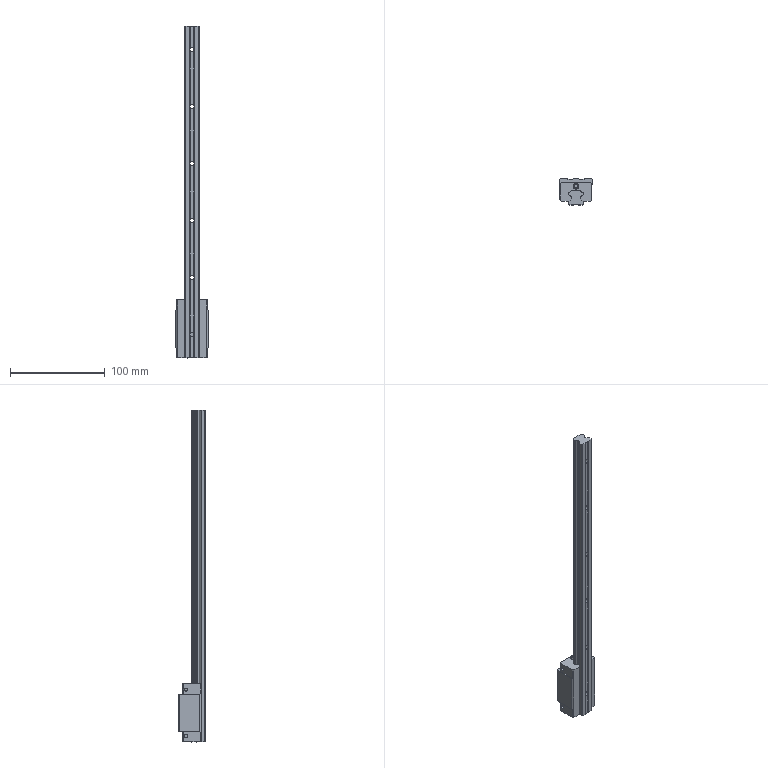Part | SolidWorks | 2 solids | 186 faces | box 34 x 28 x 350 mm | volume 100093 mm3 | plane 106 | cylinder 80 | commonest cylinder face diameters 0.8 x16 4 x12 4.5 x12 7.5 x12 3.24 x8 3.3 x8